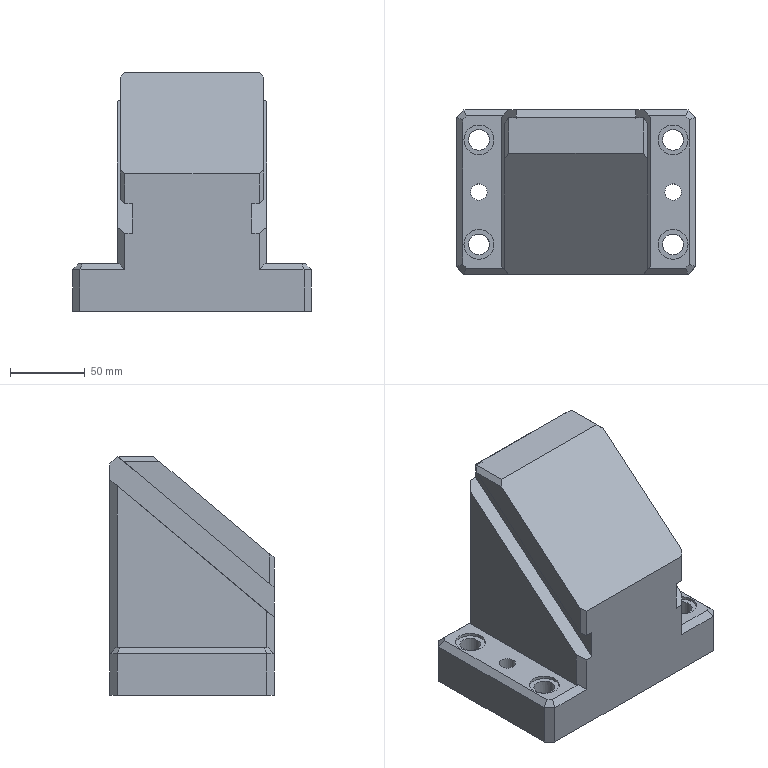Part | NX | features solid 2 | 1 solid | 63 faces | box 160 x 110 x 160 mm | volume 1517880 mm3 | plane 53 | cylinder 10 | commonest cylinder face diameters 14 x4 20 x4 11 x2